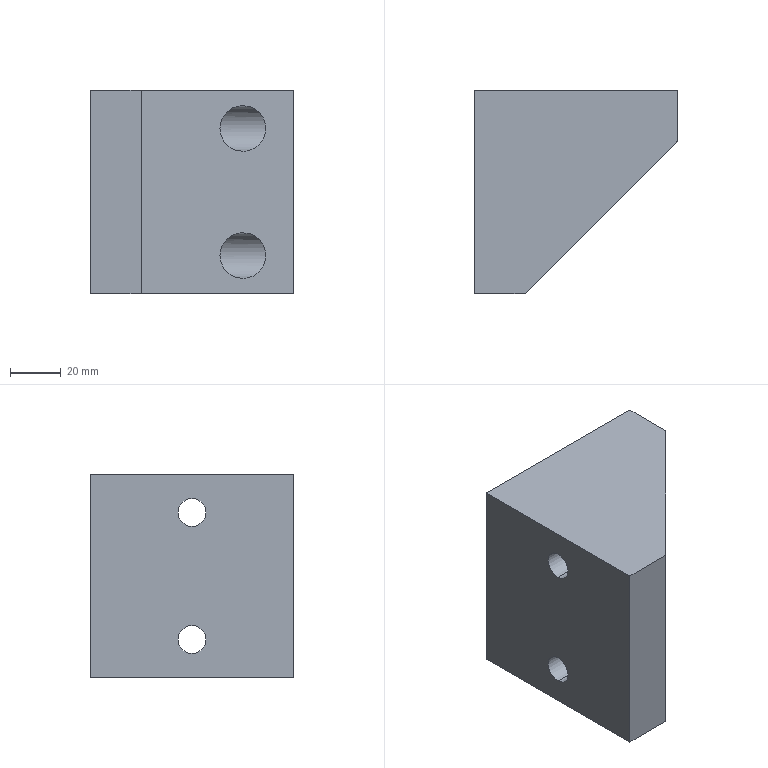Part | SolidWorks | features Extrusion 1, HoleWzd 1, ICE 1 | 1 solid | 17 faces | box 80 x 80 x 80 mm | volume 347031 mm3 | plane 9 | cylinder 8 | commonest cylinder face diameters 11 x4 18 x4
STEP:
#1=CARTESIAN_POINT('',(0.,0.,30.5));
#2=VERTEX_POINT('',#1);
#3=CARTESIAN_POINT('',(0.,0.,19.5));
#4=VERTEX_POINT('',#3);
#5=CARTESIAN_POINT('',(0.,0.,25.));
#6=DIRECTION('',(1.,0.,0.));
#7=DIRECTION('',(0.,0.,-1.));
#8=AXIS2_PLACEMENT_3D('',#5,#6,#7);
#9=CIRCLE('',#8,5.5);
#10=EDGE_CURVE('',#2,#4,#9,.T.);
#11=ORIENTED_EDGE('',*,*,#10,.F.);
#12=CARTESIAN_POINT('',(30.,0.,30.5));
#13=VERTEX_POINT('',#12);
#14=CARTESIAN_POINT('',(80.,0.,30.5));
#15=DIRECTION('',(1.,0.,0.));
#16=VECTOR('',#15,1000.);
#17=LINE('',#14,#16);
#18=EDGE_CURVE('',#2,#13,#17,.T.);
#19=ORIENTED_EDGE('',*,*,#18,.T.);
#20=CARTESIAN_POINT('',(30.,0.,19.5));
#21=VERTEX_POINT('',#20);
#22=CARTESIAN_POINT('',(30.,0.,25.));
#23=DIRECTION('',(1.,0.,0.));
#24=DIRECTION('',(0.,0.,-1.));
#25=AXIS2_PLACEMENT_3D('',#22,#23,#24);
#26=CIRCLE('',#25,5.5);
#27=EDGE_CURVE('',#13,#21,#26,.T.);
#28=ORIENTED_EDGE('',*,*,#27,.T.);
#29=CARTESIAN_POINT('',(80.,0.,19.5));
#30=DIRECTION('',(1.,0.,0.));
#31=VECTOR('',#30,1000.);
#32=LINE('',#29,#31);
#33=EDGE_CURVE('',#4,#21,#32,.T.);
#34=ORIENTED_EDGE('',*,*,#33,.F.);
#35=EDGE_LOOP('',(#11,#19,#28,#34));
#36=FACE_OUTER_BOUND('',#35,.T.);
#37=CARTESIAN_POINT('',(80.,0.,25.));
#38=DIRECTION('',(1.,0.,0.));
#39=DIRECTION('',(0.,0.,-1.));
#40=AXIS2_PLACEMENT_3D('',#37,#38,#39);
#41=CYLINDRICAL_SURFACE('',#40,5.5);
#42=ADVANCED_FACE('',(#36),#41,.F.);
#43=CARTESIAN_POINT('',(0.,0.,-19.5));
#44=VERTEX_POINT('',#43);
#45=CARTESIAN_POINT('',(0.,0.,-30.5));
#46=VERTEX_POINT('',#45);
#47=CARTESIAN_POINT('',(0.,0.,-25.));
#48=DIRECTION('',(1.,0.,0.));
#49=DIRECTION('',(0.,0.,-1.));
#50=AXIS2_PLACEMENT_3D('',#47,#48,#49);
#51=CIRCLE('',#50,5.5);
#52=EDGE_CURVE('',#44,#46,#51,.T.);
#53=ORIENTED_EDGE('',*,*,#52,.F.);
#54=CARTESIAN_POINT('',(30.,0.,-19.5));
#55=VERTEX_POINT('',#54);
#56=CARTESIAN_POINT('',(80.,0.,-19.5));
#57=DIRECTION('',(1.,0.,0.));
#58=VECTOR('',#57,1000.);
#59=LINE('',#56,#58);
#60=EDGE_CURVE('',#44,#55,#59,.T.);
#61=ORIENTED_EDGE('',*,*,#60,.T.);
#62=CARTESIAN_POINT('',(30.,0.,-30.5));
#63=VERTEX_POINT('',#62);
#64=CARTESIAN_POINT('',(30.,0.,-25.));
#65=DIRECTION('',(1.,0.,0.));
#66=DIRECTION('',(0.,0.,-1.));
#67=AXIS2_PLACEMENT_3D('',#64,#65,#66);
#68=CIRCLE('',#67,5.5);
#69=EDGE_CURVE('',#55,#63,#68,.T.);
#70=ORIENTED_EDGE('',*,*,#69,.T.);
#71=CARTESIAN_POINT('',(80.,0.,-30.5));
#72=DIRECTION('',(1.,0.,0.));
#73=VECTOR('',#72,1000.);
#74=LINE('',#71,#73);
#75=EDGE_CURVE('',#46,#63,#74,.T.);
#76=ORIENTED_EDGE('',*,*,#75,.F.);
#77=EDGE_LOOP('',(#53,#61,#70,#76));
#78=FACE_OUTER_BOUND('',#77,.T.);
#79=CARTESIAN_POINT('',(80.,0.,-25.));
#80=DIRECTION('',(1.,0.,0.));
#81=DIRECTION('',(0.,0.,-1.));
#82=AXIS2_PLACEMENT_3D('',#79,#80,#81);
#83=CYLINDRICAL_SURFACE('',#82,5.5);
#84=ADVANCED_FACE('',(#78),#83,.F.);
#85=CARTESIAN_POINT('',(30.,0.,34.));
#86=VERTEX_POINT('',#85);
#87=CARTESIAN_POINT('',(30.,0.,16.));
#88=VERTEX_POINT('',#87);
#89=CARTESIAN_POINT('',(30.,0.,25.));
#90=DIRECTION('',(1.,0.,0.));
#91=DIRECTION('',(0.,0.,-1.));
#92=AXIS2_PLACEMENT_3D('',#89,#90,#91);
#93=CIRCLE('',#92,9.);
#94=EDGE_CURVE('',#86,#88,#93,.T.);
#95=ORIENTED_EDGE('',*,*,#94,.F.);
#96=CARTESIAN_POINT('',(60.,0.,34.));
#97=VERTEX_POINT('',#96);
#98=CARTESIAN_POINT('',(80.,0.,34.));
#99=DIRECTION('',(1.,0.,0.));
#100=VECTOR('',#99,1000.);
#101=LINE('',#98,#100);
#102=EDGE_CURVE('',#86,#97,#101,.T.);
#103=ORIENTED_EDGE('',*,*,#102,.T.);
#104=CARTESIAN_POINT('',(60.,0.,16.));
#105=VERTEX_POINT('',#104);
#106=CARTESIAN_POINT('',(60.,0.,16.));
#107=CARTESIAN_POINT('',(42.,-18.,16.));
#108=CARTESIAN_POINT('',(42.,-18.,34.));
#109=CARTESIAN_POINT('',(60.,0.,34.));
#110=(BOUNDED_CURVE()B_SPLINE_CURVE(3,(#106,#107,#108,#109),.UNSPECIFIED.,.F.,.F.)B_SPLINE_CURVE_WITH_KNOTS((4,4),(1.571,4.712),.UNSPECIFIED.)CURVE()GEOMETRIC_REPRESENTATION_ITEM()RATIONAL_B_SPLINE_CURVE((1.,0.3333,0.3333,1.))REPRESENTATION_ITEM(''));
#111=EDGE_CURVE('',#105,#97,#110,.T.);
#112=ORIENTED_EDGE('',*,*,#111,.F.);
#113=CARTESIAN_POINT('',(80.,0.,16.));
#114=DIRECTION('',(1.,0.,0.));
#115=VECTOR('',#114,1000.);
#116=LINE('',#113,#115);
#117=EDGE_CURVE('',#88,#105,#116,.T.);
#118=ORIENTED_EDGE('',*,*,#117,.F.);
#119=EDGE_LOOP('',(#95,#103,#112,#118));
#120=FACE_OUTER_BOUND('',#119,.T.);
#121=CARTESIAN_POINT('',(80.,0.,25.));
#122=DIRECTION('',(1.,0.,0.));
#123=DIRECTION('',(0.,0.,-1.));
#124=AXIS2_PLACEMENT_3D('',#121,#122,#123);
#125=CYLINDRICAL_SURFACE('',#124,9.);
#126=ADVANCED_FACE('',(#120),#125,.F.);
#127=CARTESIAN_POINT('',(30.,0.,-16.));
#128=VERTEX_POINT('',#127);
#129=CARTESIAN_POINT('',(30.,0.,-34.));
#130=VERTEX_POINT('',#129);
#131=CARTESIAN_POINT('',(30.,0.,-25.));
#132=DIRECTION('',(1.,0.,0.));
#133=DIRECTION('',(0.,0.,-1.));
#134=AXIS2_PLACEMENT_3D('',#131,#132,#133);
#135=CIRCLE('',#134,9.);
#136=EDGE_CURVE('',#128,#130,#135,.T.);
#137=ORIENTED_EDGE('',*,*,#136,.F.);
#138=CARTESIAN_POINT('',(60.,0.,-16.));
#139=VERTEX_POINT('',#138);
#140=CARTESIAN_POINT('',(80.,0.,-16.));
#141=DIRECTION('',(1.,0.,0.));
#142=VECTOR('',#141,1000.);
#143=LINE('',#140,#142);
#144=EDGE_CURVE('',#128,#139,#143,.T.);
#145=ORIENTED_EDGE('',*,*,#144,.T.);
#146=CARTESIAN_POINT('',(60.,0.,-34.));
#147=VERTEX_POINT('',#146);
#148=CARTESIAN_POINT('',(60.,0.,-34.));
#149=CARTESIAN_POINT('',(42.,-18.,-34.));
#150=CARTESIAN_POINT('',(42.,-18.,-16.));
#151=CARTESIAN_POINT('',(60.,0.,-16.));
#152=(BOUNDED_CURVE()B_SPLINE_CURVE(3,(#148,#149,#150,#151),.UNSPECIFIED.,.F.,.T.)B_SPLINE_CURVE_WITH_KNOTS((4,4),(1.571,4.712),.UNSPECIFIED.)CURVE()GEOMETRIC_REPRESENTATION_ITEM()RATIONAL_B_SPLINE_CURVE((1.,0.3333,0.3333,1.))REPRESENTATION_ITEM(''));
#153=EDGE_CURVE('',#147,#139,#152,.T.);
#154=ORIENTED_EDGE('',*,*,#153,.F.);
#155=CARTESIAN_POINT('',(80.,0.,-34.));
#156=DIRECTION('',(1.,0.,0.));
#157=VECTOR('',#156,1000.);
#158=LINE('',#155,#157);
#159=EDGE_CURVE('',#130,#147,#158,.T.);
#160=ORIENTED_EDGE('',*,*,#159,.F.);
#161=EDGE_LOOP('',(#137,#145,#154,#160));
#162=FACE_OUTER_BOUND('',#161,.T.);
#163=CARTESIAN_POINT('',(80.,0.,-25.));
#164=DIRECTION('',(1.,0.,0.));
#165=DIRECTION('',(0.,0.,-1.));
#166=AXIS2_PLACEMENT_3D('',#163,#164,#165);
#167=CYLINDRICAL_SURFACE('',#166,9.);
#168=ADVANCED_FACE('',(#162),#167,.F.);
#169=CARTESIAN_POINT('',(20.,-40.,-40.));
#170=VERTEX_POINT('',#169);
#171=CARTESIAN_POINT('',(80.,20.,-40.));
#172=VERTEX_POINT('',#171);
#173=CARTESIAN_POINT('',(20.,-40.,-40.));
#174=DIRECTION('',(0.7071,0.7071,0.));
#175=VECTOR('',#174,1000.);
#176=LINE('',#173,#175);
#177=EDGE_CURVE('',#170,#172,#176,.T.);
#178=ORIENTED_EDGE('',*,*,#177,.F.);
#179=CARTESIAN_POINT('',(0.,-40.,-40.));
#180=VERTEX_POINT('',#179);
#181=CARTESIAN_POINT('',(80.,-40.,-40.));
#182=DIRECTION('',(-1.,0.,0.));
#183=VECTOR('',#182,1000.);
#184=LINE('',#181,#183);
#185=EDGE_CURVE('',#170,#180,#184,.T.);
#186=ORIENTED_EDGE('',*,*,#185,.T.);
#187=CARTESIAN_POINT('',(0.,40.,-40.));
#188=VERTEX_POINT('',#187);
#189=CARTESIAN_POINT('',(0.,40.,-40.));
#190=DIRECTION('',(0.,1.,0.));
#191=VECTOR('',#190,1000.);
#192=LINE('',#189,#191);
#193=EDGE_CURVE('',#180,#188,#192,.T.);
#194=ORIENTED_EDGE('',*,*,#193,.T.);
#195=CARTESIAN_POINT('',(80.,40.,-40.));
#196=VERTEX_POINT('',#195);
#197=CARTESIAN_POINT('',(80.,40.,-40.));
#198=DIRECTION('',(-1.,0.,0.));
#199=VECTOR('',#198,1000.);
#200=LINE('',#197,#199);
#201=EDGE_CURVE('',#196,#188,#200,.T.);
#202=ORIENTED_EDGE('',*,*,#201,.F.);
#203=CARTESIAN_POINT('',(80.,40.,-40.));
#204=DIRECTION('',(0.,1.,0.));
#205=VECTOR('',#204,1000.);
#206=LINE('',#203,#205);
#207=EDGE_CURVE('',#172,#196,#206,.T.);
#208=ORIENTED_EDGE('',*,*,#207,.F.);
#209=EDGE_LOOP('',(#178,#186,#194,#202,#208));
#210=FACE_OUTER_BOUND('',#209,.T.);
#211=CARTESIAN_POINT('',(80.,40.,-40.));
#212=DIRECTION('',(0.,0.,1.));
#213=DIRECTION('',(0.,-1.,0.));
#214=AXIS2_PLACEMENT_3D('',#211,#212,#213);
#215=PLANE('',#214);
#216=ADVANCED_FACE('',(#210),#215,.F.);
#217=CARTESIAN_POINT('',(20.,-40.,40.));
#218=VERTEX_POINT('',#217);
#219=CARTESIAN_POINT('',(80.,20.,40.));
#220=VERTEX_POINT('',#219);
#221=CARTESIAN_POINT('',(20.,-40.,40.));
#222=DIRECTION('',(0.7071,0.7071,0.));
#223=VECTOR('',#222,1000.);
#224=LINE('',#221,#223);
#225=EDGE_CURVE('',#218,#220,#224,.T.);
#226=ORIENTED_EDGE('',*,*,#225,.T.);
#227=CARTESIAN_POINT('',(80.,40.,40.));
#228=VERTEX_POINT('',#227);
#229=CARTESIAN_POINT('',(80.,40.,40.));
#230=DIRECTION('',(0.,-1.,0.));
#231=VECTOR('',#230,1000.);
#232=LINE('',#229,#231);
#233=EDGE_CURVE('',#228,#220,#232,.T.);
#234=ORIENTED_EDGE('',*,*,#233,.F.);
#235=CARTESIAN_POINT('',(0.,40.,40.));
#236=VERTEX_POINT('',#235);
#237=CARTESIAN_POINT('',(80.,40.,40.));
#238=DIRECTION('',(-1.,0.,0.));
#239=VECTOR('',#238,1000.);
#240=LINE('',#237,#239);
#241=EDGE_CURVE('',#228,#236,#240,.T.);
#242=ORIENTED_EDGE('',*,*,#241,.T.);
#243=CARTESIAN_POINT('',(0.,-40.,40.));
#244=VERTEX_POINT('',#243);
#245=CARTESIAN_POINT('',(0.,40.,40.));
#246=DIRECTION('',(0.,-1.,0.));
#247=VECTOR('',#246,1000.);
#248=LINE('',#245,#247);
#249=EDGE_CURVE('',#236,#244,#248,.T.);
#250=ORIENTED_EDGE('',*,*,#249,.T.);
#251=CARTESIAN_POINT('',(80.,-40.,40.));
#252=DIRECTION('',(-1.,0.,0.));
#253=VECTOR('',#252,1000.);
#254=LINE('',#251,#253);
#255=EDGE_CURVE('',#218,#244,#254,.T.);
#256=ORIENTED_EDGE('',*,*,#255,.F.);
#257=EDGE_LOOP('',(#226,#234,#242,#250,#256));
#258=FACE_OUTER_BOUND('',#257,.T.);
#259=CARTESIAN_POINT('',(80.,40.,40.));
#260=DIRECTION('',(0.,0.,-1.));
#261=DIRECTION('',(0.,1.,0.));
#262=AXIS2_PLACEMENT_3D('',#259,#260,#261);
#263=PLANE('',#262);
#264=ADVANCED_FACE('',(#258),#263,.F.);
#265=CARTESIAN_POINT('',(20.,-40.,-40.));
#266=DIRECTION('',(0.,0.,1.));
#267=VECTOR('',#266,1000.);
#268=LINE('',#265,#267);
#269=EDGE_CURVE('',#170,#218,#268,.T.);
#270=ORIENTED_EDGE('',*,*,#269,.T.);
#271=ORIENTED_EDGE('',*,*,#255,.T.);
#272=CARTESIAN_POINT('',(0.,-40.,40.));
#273=DIRECTION('',(0.,0.,-1.));
#274=VECTOR('',#273,1000.);
#275=LINE('',#272,#274);
#276=EDGE_CURVE('',#244,#180,#275,.T.);
#277=ORIENTED_EDGE('',*,*,#276,.T.);
#278=ORIENTED_EDGE('',*,*,#185,.F.);
#279=EDGE_LOOP('',(#270,#271,#277,#278));
#280=FACE_OUTER_BOUND('',#279,.T.);
#281=CARTESIAN_POINT('',(80.,-40.,40.));
#282=DIRECTION('',(0.,1.,0.));
#283=DIRECTION('',(0.,0.,1.));
#284=AXIS2_PLACEMENT_3D('',#281,#282,#283);
#285=PLANE('',#284);
#286=ADVANCED_FACE('',(#280),#285,.F.);
#287=ORIENTED_EDGE('',*,*,#233,.T.);
#288=CARTESIAN_POINT('',(80.,20.,-40.));
#289=DIRECTION('',(0.,0.,1.));
#290=VECTOR('',#289,1000.);
#291=LINE('',#288,#290);
#292=EDGE_CURVE('',#172,#220,#291,.T.);
#293=ORIENTED_EDGE('',*,*,#292,.F.);
#294=ORIENTED_EDGE('',*,*,#207,.T.);
#295=CARTESIAN_POINT('',(80.,40.,40.));
#296=DIRECTION('',(0.,0.,1.));
#297=VECTOR('',#296,1000.);
#298=LINE('',#295,#297);
#299=EDGE_CURVE('',#196,#228,#298,.T.);
#300=ORIENTED_EDGE('',*,*,#299,.T.);
#301=EDGE_LOOP('',(#287,#293,#294,#300));
#302=FACE_OUTER_BOUND('',#301,.T.);
#303=CARTESIAN_POINT('',(80.,0.,0.));
#304=DIRECTION('',(1.,0.,0.));
#305=DIRECTION('',(0.,0.,-1.));
#306=AXIS2_PLACEMENT_3D('',#303,#304,#305);
#307=PLANE('',#306);
#308=ADVANCED_FACE('',(#302),#307,.T.);
#309=ORIENTED_EDGE('',*,*,#144,.F.);
#310=CARTESIAN_POINT('',(30.,0.,-25.));
#311=DIRECTION('',(1.,0.,0.));
#312=DIRECTION('',(0.,0.,-1.));
#313=AXIS2_PLACEMENT_3D('',#310,#311,#312);
#314=CIRCLE('',#313,9.);
#315=EDGE_CURVE('',#130,#128,#314,.T.);
#316=ORIENTED_EDGE('',*,*,#315,.F.);
#317=ORIENTED_EDGE('',*,*,#159,.T.);
#318=CARTESIAN_POINT('',(60.,0.,-16.));
#319=CARTESIAN_POINT('',(78.,18.,-16.));
#320=CARTESIAN_POINT('',(78.,18.,-34.));
#321=CARTESIAN_POINT('',(60.,0.,-34.));
#322=(BOUNDED_CURVE()B_SPLINE_CURVE(3,(#318,#319,#320,#321),.UNSPECIFIED.,.F.,.F.)B_SPLINE_CURVE_WITH_KNOTS((4,4),(4.712,7.854),.UNSPECIFIED.)CURVE()GEOMETRIC_REPRESENTATION_ITEM()RATIONAL_B_SPLINE_CURVE((1.,0.3333,0.3333,1.))REPRESENTATION_ITEM(''));
#323=EDGE_CURVE('',#139,#147,#322,.T.);
#324=ORIENTED_EDGE('',*,*,#323,.F.);
#325=EDGE_LOOP('',(#309,#316,#317,#324));
#326=FACE_OUTER_BOUND('',#325,.T.);
#327=CARTESIAN_POINT('',(80.,0.,-25.));
#328=DIRECTION('',(1.,0.,0.));
#329=DIRECTION('',(0.,0.,-1.));
#330=AXIS2_PLACEMENT_3D('',#327,#328,#329);
#331=CYLINDRICAL_SURFACE('',#330,9.);
#332=ADVANCED_FACE('',(#326),#331,.F.);
#333=ORIENTED_EDGE('',*,*,#102,.F.);
#334=CARTESIAN_POINT('',(30.,0.,25.));
#335=DIRECTION('',(1.,0.,0.));
#336=DIRECTION('',(0.,0.,-1.));
#337=AXIS2_PLACEMENT_3D('',#334,#335,#336);
#338=CIRCLE('',#337,9.);
#339=EDGE_CURVE('',#88,#86,#338,.T.);
#340=ORIENTED_EDGE('',*,*,#339,.F.);
#341=ORIENTED_EDGE('',*,*,#117,.T.);
#342=CARTESIAN_POINT('',(60.,0.,34.));
#343=CARTESIAN_POINT('',(78.,18.,34.));
#344=CARTESIAN_POINT('',(78.,18.,16.));
#345=CARTESIAN_POINT('',(60.,0.,16.));
#346=(BOUNDED_CURVE()B_SPLINE_CURVE(3,(#342,#343,#344,#345),.UNSPECIFIED.,.F.,.F.)B_SPLINE_CURVE_WITH_KNOTS((4,4),(4.712,7.854),.UNSPECIFIED.)CURVE()GEOMETRIC_REPRESENTATION_ITEM()RATIONAL_B_SPLINE_CURVE((1.,0.3333,0.3333,1.))REPRESENTATION_ITEM(''));
#347=EDGE_CURVE('',#97,#105,#346,.T.);
#348=ORIENTED_EDGE('',*,*,#347,.F.);
#349=EDGE_LOOP('',(#333,#340,#341,#348));
#350=FACE_OUTER_BOUND('',#349,.T.);
#351=CARTESIAN_POINT('',(80.,0.,25.));
#352=DIRECTION('',(1.,0.,0.));
#353=DIRECTION('',(0.,0.,-1.));
#354=AXIS2_PLACEMENT_3D('',#351,#352,#353);
#355=CYLINDRICAL_SURFACE('',#354,9.);
#356=ADVANCED_FACE('',(#350),#355,.F.);
#357=CARTESIAN_POINT('',(0.,40.,40.));
#358=DIRECTION('',(0.,0.,1.));
#359=VECTOR('',#358,1000.);
#360=LINE('',#357,#359);
#361=EDGE_CURVE('',#188,#236,#360,.T.);
#362=ORIENTED_EDGE('',*,*,#361,.T.);
#363=ORIENTED_EDGE('',*,*,#241,.F.);
#364=ORIENTED_EDGE('',*,*,#299,.F.);
#365=ORIENTED_EDGE('',*,*,#201,.T.);
#366=EDGE_LOOP('',(#362,#363,#364,#365));
#367=FACE_OUTER_BOUND('',#366,.T.);
#368=CARTESIAN_POINT('',(80.,40.,40.));
#369=DIRECTION('',(0.,-1.,0.));
#370=DIRECTION('',(0.,0.,-1.));
#371=AXIS2_PLACEMENT_3D('',#368,#369,#370);
#372=PLANE('',#371);
#373=ADVANCED_FACE('',(#367),#372,.F.);
#374=CARTESIAN_POINT('',(0.,0.,25.));
#375=DIRECTION('',(1.,0.,0.));
#376=DIRECTION('',(0.,0.,-1.));
#377=AXIS2_PLACEMENT_3D('',#374,#375,#376);
#378=CIRCLE('',#377,5.5);
#379=EDGE_CURVE('',#4,#2,#378,.T.);
#380=ORIENTED_EDGE('',*,*,#379,.T.);
#381=ORIENTED_EDGE('',*,*,#10,.T.);
#382=EDGE_LOOP('',(#380,#381));
#383=FACE_BOUND('',#382,.T.);
#384=CARTESIAN_POINT('',(0.,0.,-25.));
#385=DIRECTION('',(1.,0.,0.));
#386=DIRECTION('',(0.,0.,-1.));
#387=AXIS2_PLACEMENT_3D('',#384,#385,#386);
#388=CIRCLE('',#387,5.5);
#389=EDGE_CURVE('',#46,#44,#388,.T.);
#390=ORIENTED_EDGE('',*,*,#389,.T.);
#391=ORIENTED_EDGE('',*,*,#52,.T.);
#392=EDGE_LOOP('',(#390,#391));
#393=FACE_BOUND('',#392,.T.);
#394=ORIENTED_EDGE('',*,*,#193,.F.);
#395=ORIENTED_EDGE('',*,*,#276,.F.);
#396=ORIENTED_EDGE('',*,*,#249,.F.);
#397=ORIENTED_EDGE('',*,*,#361,.F.);
#398=EDGE_LOOP('',(#394,#395,#396,#397));
#399=FACE_OUTER_BOUND('',#398,.T.);
#400=CARTESIAN_POINT('',(0.,0.,0.));
#401=DIRECTION('',(1.,0.,0.));
#402=DIRECTION('',(0.,0.,-1.));
#403=AXIS2_PLACEMENT_3D('',#400,#401,#402);
#404=PLANE('',#403);
#405=ADVANCED_FACE('',(#383,#393,#399),#404,.F.);
#406=ORIENTED_EDGE('',*,*,#60,.F.);
#407=ORIENTED_EDGE('',*,*,#389,.F.);
#408=ORIENTED_EDGE('',*,*,#75,.T.);
#409=CARTESIAN_POINT('',(30.,0.,-25.));
#410=DIRECTION('',(1.,0.,0.));
#411=DIRECTION('',(0.,0.,-1.));
#412=AXIS2_PLACEMENT_3D('',#409,#410,#411);
#413=CIRCLE('',#412,5.5);
#414=EDGE_CURVE('',#63,#55,#413,.T.);
#415=ORIENTED_EDGE('',*,*,#414,.T.);
#416=EDGE_LOOP('',(#406,#407,#408,#415));
#417=FACE_OUTER_BOUND('',#416,.T.);
#418=CARTESIAN_POINT('',(80.,0.,-25.));
#419=DIRECTION('',(1.,0.,0.));
#420=DIRECTION('',(0.,0.,-1.));
#421=AXIS2_PLACEMENT_3D('',#418,#419,#420);
#422=CYLINDRICAL_SURFACE('',#421,5.5);
#423=ADVANCED_FACE('',(#417),#422,.F.);
#424=ORIENTED_EDGE('',*,*,#414,.F.);
#425=ORIENTED_EDGE('',*,*,#69,.F.);
#426=EDGE_LOOP('',(#424,#425));
#427=FACE_BOUND('',#426,.T.);
#428=ORIENTED_EDGE('',*,*,#315,.T.);
#429=ORIENTED_EDGE('',*,*,#136,.T.);
#430=EDGE_LOOP('',(#428,#429));
#431=FACE_OUTER_BOUND('',#430,.T.);
#432=CARTESIAN_POINT('',(30.,5.5,-25.));
#433=DIRECTION('',(-1.,0.,0.));
#434=DIRECTION('',(0.,0.,1.));
#435=AXIS2_PLACEMENT_3D('',#432,#433,#434);
#436=PLANE('',#435);
#437=ADVANCED_FACE('',(#427,#431),#436,.F.);
#438=ORIENTED_EDGE('',*,*,#18,.F.);
#439=ORIENTED_EDGE('',*,*,#379,.F.);
#440=ORIENTED_EDGE('',*,*,#33,.T.);
#441=CARTESIAN_POINT('',(30.,0.,25.));
#442=DIRECTION('',(1.,0.,0.));
#443=DIRECTION('',(0.,0.,-1.));
#444=AXIS2_PLACEMENT_3D('',#441,#442,#443);
#445=CIRCLE('',#444,5.5);
#446=EDGE_CURVE('',#21,#13,#445,.T.);
#447=ORIENTED_EDGE('',*,*,#446,.T.);
#448=EDGE_LOOP('',(#438,#439,#440,#447));
#449=FACE_OUTER_BOUND('',#448,.T.);
#450=CARTESIAN_POINT('',(80.,0.,25.));
#451=DIRECTION('',(1.,0.,0.));
#452=DIRECTION('',(0.,0.,-1.));
#453=AXIS2_PLACEMENT_3D('',#450,#451,#452);
#454=CYLINDRICAL_SURFACE('',#453,5.5);
#455=ADVANCED_FACE('',(#449),#454,.F.);
#456=ORIENTED_EDGE('',*,*,#446,.F.);
#457=ORIENTED_EDGE('',*,*,#27,.F.);
#458=EDGE_LOOP('',(#456,#457));
#459=FACE_BOUND('',#458,.T.);
#460=ORIENTED_EDGE('',*,*,#339,.T.);
#461=ORIENTED_EDGE('',*,*,#94,.T.);
#462=EDGE_LOOP('',(#460,#461));
#463=FACE_OUTER_BOUND('',#462,.T.);
#464=CARTESIAN_POINT('',(30.,5.5,25.));
#465=DIRECTION('',(-1.,0.,0.));
#466=DIRECTION('',(0.,0.,1.));
#467=AXIS2_PLACEMENT_3D('',#464,#465,#466);
#468=PLANE('',#467);
#469=ADVANCED_FACE('',(#459,#463),#468,.F.);
#470=ORIENTED_EDGE('',*,*,#225,.F.);
#471=ORIENTED_EDGE('',*,*,#269,.F.);
#472=ORIENTED_EDGE('',*,*,#177,.T.);
#473=ORIENTED_EDGE('',*,*,#292,.T.);
#474=EDGE_LOOP('',(#470,#471,#472,#473));
#475=FACE_OUTER_BOUND('',#474,.T.);
#476=ORIENTED_EDGE('',*,*,#111,.T.);
#477=ORIENTED_EDGE('',*,*,#347,.T.);
#478=EDGE_LOOP('',(#476,#477));
#479=FACE_BOUND('',#478,.T.);
#480=ORIENTED_EDGE('',*,*,#153,.T.);
#481=ORIENTED_EDGE('',*,*,#323,.T.);
#482=EDGE_LOOP('',(#480,#481));
#483=FACE_BOUND('',#482,.T.);
#484=CARTESIAN_POINT('',(20.,-40.,-40.));
#485=DIRECTION('',(0.7071,-0.7071,0.));
#486=DIRECTION('',(0.7071,0.7071,0.));
#487=AXIS2_PLACEMENT_3D('',#484,#485,#486);
#488=PLANE('',#487);
#489=ADVANCED_FACE('',(#475,#479,#483),#488,.T.);
#490=CLOSED_SHELL('',(#42,#84,#126,#168,#216,#264,#286,#308,#332,#356,#373,#405,#423,#437,#455,#469,#489));
#491=MANIFOLD_SOLID_BREP('',#490);
#492=CARTESIAN_POINT('',(0.,0.,0.));
#493=DIRECTION('',(0.,0.,1.));
#494=DIRECTION('',(1.,0.,0.));
#495=AXIS2_PLACEMENT_3D('',#492,#493,#494);
#496=(LENGTH_UNIT()NAMED_UNIT(*)SI_UNIT(.MILLI.,.METRE.));
#497=UNCERTAINTY_MEASURE_WITH_UNIT(LENGTH_MEASURE(0.00001),#496,'','');
#498=(NAMED_UNIT(*)PLANE_ANGLE_UNIT()SI_UNIT($,.RADIAN.));
#499=(NAMED_UNIT(*)SI_UNIT($,.STERADIAN.)SOLID_ANGLE_UNIT());
#500=(GEOMETRIC_REPRESENTATION_CONTEXT(3)GLOBAL_UNCERTAINTY_ASSIGNED_CONTEXT((#497))GLOBAL_UNIT_ASSIGNED_CONTEXT((#496,#498,#499))REPRESENTATION_CONTEXT('',''));
#501=ADVANCED_BREP_SHAPE_REPRESENTATION('',(#491,#495),#500);